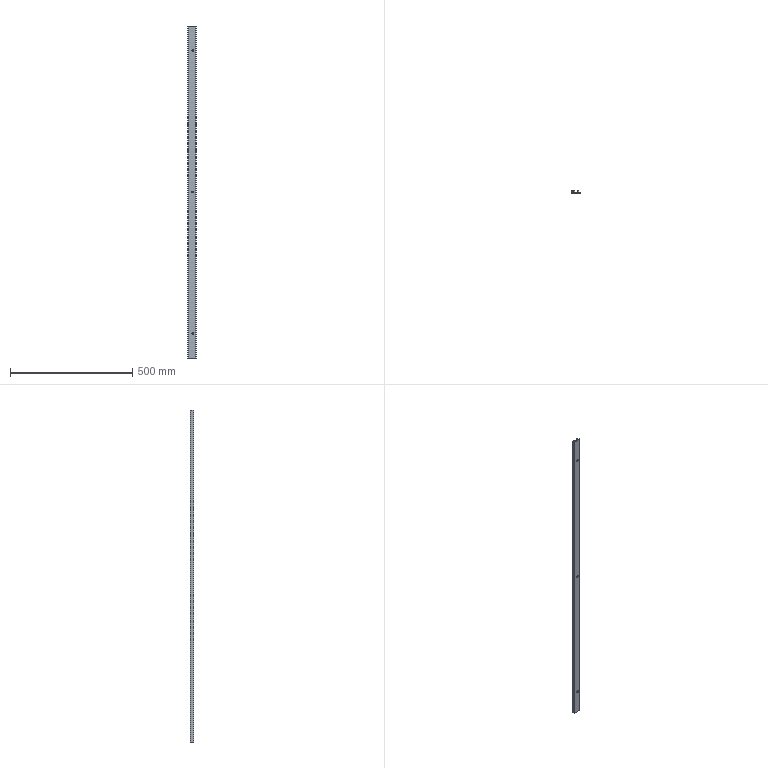Part | 1 solid | 31 faces | box 33.5 x 13.5 x 1360 mm | volume 254381 mm3 | plane 16 | cylinder 9 | cone 6 | commonest cylinder face diameters 2 x3 13.44 x3 4 x2 1.5 x1
STEP:
#1=CARTESIAN_POINT('',(20.,0.,1163.72));
#2=VERTEX_POINT('',#1);
#3=CARTESIAN_POINT('',(20.,0.,1156.28));
#4=VERTEX_POINT('',#3);
#5=CARTESIAN_POINT('',(20.,0.,1160.));
#6=DIRECTION('',(0.,-1.,0.));
#7=DIRECTION('',(0.,0.,-1.));
#8=AXIS2_PLACEMENT_3D('',#5,#6,#7);
#9=CIRCLE('',#8,3.72);
#10=EDGE_CURVE('',#2,#4,#9,.T.);
#11=ORIENTED_EDGE('',*,*,#10,.T.);
#12=CARTESIAN_POINT('',(20.,3.,1153.28));
#13=VERTEX_POINT('',#12);
#14=CARTESIAN_POINT('',(20.,3.,1153.28));
#15=DIRECTION('',(0.,0.7071,-0.7071));
#16=VECTOR('',#15,1000.);
#17=LINE('',#14,#16);
#18=EDGE_CURVE('',#4,#13,#17,.T.);
#19=ORIENTED_EDGE('',*,*,#18,.T.);
#20=CARTESIAN_POINT('',(20.,3.,1166.72));
#21=VERTEX_POINT('',#20);
#22=CARTESIAN_POINT('',(20.,3.,1160.));
#23=DIRECTION('',(0.,1.,0.));
#24=DIRECTION('',(0.,0.,1.));
#25=AXIS2_PLACEMENT_3D('',#22,#23,#24);
#26=CIRCLE('',#25,6.72);
#27=EDGE_CURVE('',#13,#21,#26,.T.);
#28=ORIENTED_EDGE('',*,*,#27,.T.);
#29=CARTESIAN_POINT('',(20.,3.,1166.72));
#30=DIRECTION('',(0.,0.7071,0.7071));
#31=VECTOR('',#30,1000.);
#32=LINE('',#29,#31);
#33=EDGE_CURVE('',#2,#21,#32,.T.);
#34=ORIENTED_EDGE('',*,*,#33,.F.);
#35=EDGE_LOOP('',(#11,#19,#28,#34));
#36=FACE_OUTER_BOUND('',#35,.T.);
#37=CARTESIAN_POINT('',(20.,3.,1160.));
#38=DIRECTION('',(0.,1.,0.));
#39=DIRECTION('',(0.,0.,1.));
#40=AXIS2_PLACEMENT_3D('',#37,#38,#39);
#41=CONICAL_SURFACE('',#40,6.72,0.7854);
#42=ADVANCED_FACE('',(#36),#41,.F.);
#43=CARTESIAN_POINT('',(20.,0.,3.72));
#44=VERTEX_POINT('',#43);
#45=CARTESIAN_POINT('',(20.,0.,-3.72));
#46=VERTEX_POINT('',#45);
#47=CARTESIAN_POINT('',(20.,0.,0.));
#48=DIRECTION('',(0.,-1.,0.));
#49=DIRECTION('',(0.,0.,-1.));
#50=AXIS2_PLACEMENT_3D('',#47,#48,#49);
#51=CIRCLE('',#50,3.72);
#52=EDGE_CURVE('',#44,#46,#51,.T.);
#53=ORIENTED_EDGE('',*,*,#52,.T.);
#54=CARTESIAN_POINT('',(20.,3.,-6.72));
#55=VERTEX_POINT('',#54);
#56=CARTESIAN_POINT('',(20.,3.,-6.72));
#57=DIRECTION('',(0.,0.7071,-0.7071));
#58=VECTOR('',#57,1000.);
#59=LINE('',#56,#58);
#60=EDGE_CURVE('',#46,#55,#59,.T.);
#61=ORIENTED_EDGE('',*,*,#60,.T.);
#62=CARTESIAN_POINT('',(20.,3.,6.72));
#63=VERTEX_POINT('',#62);
#64=CARTESIAN_POINT('',(20.,3.,0.));
#65=DIRECTION('',(0.,1.,0.));
#66=DIRECTION('',(0.,0.,1.));
#67=AXIS2_PLACEMENT_3D('',#64,#65,#66);
#68=CIRCLE('',#67,6.72);
#69=EDGE_CURVE('',#55,#63,#68,.T.);
#70=ORIENTED_EDGE('',*,*,#69,.T.);
#71=CARTESIAN_POINT('',(20.,3.,6.72));
#72=DIRECTION('',(0.,0.7071,0.7071));
#73=VECTOR('',#72,1000.);
#74=LINE('',#71,#73);
#75=EDGE_CURVE('',#44,#63,#74,.T.);
#76=ORIENTED_EDGE('',*,*,#75,.F.);
#77=EDGE_LOOP('',(#53,#61,#70,#76));
#78=FACE_OUTER_BOUND('',#77,.T.);
#79=CARTESIAN_POINT('',(20.,3.,0.));
#80=DIRECTION('',(0.,1.,0.));
#81=DIRECTION('',(0.,0.,1.));
#82=AXIS2_PLACEMENT_3D('',#79,#80,#81);
#83=CONICAL_SURFACE('',#82,6.72,0.7854);
#84=ADVANCED_FACE('',(#78),#83,.F.);
#85=CARTESIAN_POINT('',(20.,0.,583.72));
#86=VERTEX_POINT('',#85);
#87=CARTESIAN_POINT('',(20.,0.,576.28));
#88=VERTEX_POINT('',#87);
#89=CARTESIAN_POINT('',(20.,0.,580.));
#90=DIRECTION('',(0.,-1.,0.));
#91=DIRECTION('',(0.,0.,-1.));
#92=AXIS2_PLACEMENT_3D('',#89,#90,#91);
#93=CIRCLE('',#92,3.72);
#94=EDGE_CURVE('',#86,#88,#93,.T.);
#95=ORIENTED_EDGE('',*,*,#94,.T.);
#96=CARTESIAN_POINT('',(20.,3.,573.28));
#97=VERTEX_POINT('',#96);
#98=CARTESIAN_POINT('',(20.,3.,573.28));
#99=DIRECTION('',(0.,0.7071,-0.7071));
#100=VECTOR('',#99,1000.);
#101=LINE('',#98,#100);
#102=EDGE_CURVE('',#88,#97,#101,.T.);
#103=ORIENTED_EDGE('',*,*,#102,.T.);
#104=CARTESIAN_POINT('',(20.,3.,586.72));
#105=VERTEX_POINT('',#104);
#106=CARTESIAN_POINT('',(20.,3.,580.));
#107=DIRECTION('',(0.,1.,0.));
#108=DIRECTION('',(0.,0.,1.));
#109=AXIS2_PLACEMENT_3D('',#106,#107,#108);
#110=CIRCLE('',#109,6.72);
#111=EDGE_CURVE('',#97,#105,#110,.T.);
#112=ORIENTED_EDGE('',*,*,#111,.T.);
#113=CARTESIAN_POINT('',(20.,3.,586.72));
#114=DIRECTION('',(0.,0.7071,0.7071));
#115=VECTOR('',#114,1000.);
#116=LINE('',#113,#115);
#117=EDGE_CURVE('',#86,#105,#116,.T.);
#118=ORIENTED_EDGE('',*,*,#117,.F.);
#119=EDGE_LOOP('',(#95,#103,#112,#118));
#120=FACE_OUTER_BOUND('',#119,.T.);
#121=CARTESIAN_POINT('',(20.,3.,580.));
#122=DIRECTION('',(0.,1.,0.));
#123=DIRECTION('',(0.,0.,1.));
#124=AXIS2_PLACEMENT_3D('',#121,#122,#123);
#125=CONICAL_SURFACE('',#124,6.72,0.7854);
#126=ADVANCED_FACE('',(#120),#125,.F.);
#127=CARTESIAN_POINT('',(24.5,10.5,-4.991));
#128=VERTEX_POINT('',#127);
#129=CARTESIAN_POINT('',(24.5,10.5,-100.));
#130=VERTEX_POINT('',#129);
#131=CARTESIAN_POINT('',(24.5,10.5,-100.));
#132=DIRECTION('',(0.,0.,-1.));
#133=VECTOR('',#132,1000.);
#134=LINE('',#131,#133);
#135=EDGE_CURVE('',#128,#130,#134,.T.);
#136=ORIENTED_EDGE('',*,*,#135,.F.);
#137=CARTESIAN_POINT('',(24.5,10.5,4.991));
#138=VERTEX_POINT('',#137);
#139=CARTESIAN_POINT('',(24.5,10.5,-4.991));
#140=CARTESIAN_POINT('',(24.5,10.638,-4.991));
#141=CARTESIAN_POINT('',(24.515,10.777,-4.978));
#142=CARTESIAN_POINT('',(24.57,11.043,-4.927));
#143=CARTESIAN_POINT('',(24.611,11.171,-4.889));
#144=CARTESIAN_POINT('',(24.765,11.529,-4.74));
#145=CARTESIAN_POINT('',(24.907,11.728,-4.597));
#146=CARTESIAN_POINT('',(25.205,12.04,-4.256));
#147=CARTESIAN_POINT('',(25.365,12.156,-4.055));
#148=CARTESIAN_POINT('',(25.663,12.325,-3.627));
#149=CARTESIAN_POINT('',(25.806,12.38,-3.395));
#150=CARTESIAN_POINT('',(26.19,12.494,-2.672));
#151=CARTESIAN_POINT('',(26.387,12.501,-2.161));
#152=CARTESIAN_POINT('',(26.654,12.499,-1.091));
#153=CARTESIAN_POINT('',(26.72,12.488,-0.5481));
#154=CARTESIAN_POINT('',(26.72,12.488,0.2773));
#155=CARTESIAN_POINT('',(26.703,12.49,0.5529));
#156=CARTESIAN_POINT('',(26.636,12.496,1.095));
#157=CARTESIAN_POINT('',(26.586,12.499,1.362));
#158=CARTESIAN_POINT('',(26.388,12.501,2.155));
#159=CARTESIAN_POINT('',(26.188,12.493,2.677));
#160=CARTESIAN_POINT('',(25.805,12.38,3.396));
#161=CARTESIAN_POINT('',(25.662,12.324,3.629));
#162=CARTESIAN_POINT('',(25.438,12.197,3.95));
#163=CARTESIAN_POINT('',(25.362,12.147,4.053));
#164=CARTESIAN_POINT('',(25.208,12.03,4.249));
#165=CARTESIAN_POINT('',(25.13,11.961,4.342));
#166=CARTESIAN_POINT('',(24.98,11.805,4.513));
#167=CARTESIAN_POINT('',(24.908,11.717,4.591));
#168=CARTESIAN_POINT('',(24.774,11.518,4.73));
#169=CARTESIAN_POINT('',(24.714,11.408,4.79));
#170=CARTESIAN_POINT('',(24.612,11.172,4.888));
#171=CARTESIAN_POINT('',(24.57,11.043,4.927));
#172=CARTESIAN_POINT('',(24.515,10.778,4.978));
#173=CARTESIAN_POINT('',(24.5,10.64,4.991));
#174=CARTESIAN_POINT('',(24.5,10.5,4.991));
#175=B_SPLINE_CURVE_WITH_KNOTS('',3,(#139,#140,#141,#142,#143,#144,#145,#146,#147,#148,#149,#150,#151,#152,#153,#154,#155,#156,#157,#158,#159,#160,#161,#162,#163,#164,#165,#166,#167,#168,#169,#170,#171,#172,#173,#174),.UNSPECIFIED.,.F.,.F.,(4,2,2,2,2,2,2,2,2,2,2,2,2,2,2,2,2,4),(0.01321,0.01362,0.01403,0.01486,0.01569,0.01651,0.01816,0.01981,0.02064,0.02146,0.02311,0.02394,0.02435,0.02477,0.02518,0.02559,0.026,0.02642),.UNSPECIFIED.);
#176=EDGE_CURVE('',#128,#138,#175,.T.);
#177=ORIENTED_EDGE('',*,*,#176,.T.);
#178=CARTESIAN_POINT('',(24.5,10.5,575.009));
#179=VERTEX_POINT('',#178);
#180=CARTESIAN_POINT('',(24.5,10.5,-100.));
#181=DIRECTION('',(0.,0.,-1.));
#182=VECTOR('',#181,1000.);
#183=LINE('',#180,#182);
#184=EDGE_CURVE('',#179,#138,#183,.T.);
#185=ORIENTED_EDGE('',*,*,#184,.F.);
#186=CARTESIAN_POINT('',(24.5,10.5,584.991));
#187=VERTEX_POINT('',#186);
#188=CARTESIAN_POINT('',(24.5,10.5,575.009));
#189=CARTESIAN_POINT('',(24.5,10.638,575.009));
#190=CARTESIAN_POINT('',(24.515,10.777,575.022));
#191=CARTESIAN_POINT('',(24.57,11.043,575.073));
#192=CARTESIAN_POINT('',(24.611,11.171,575.111));
#193=CARTESIAN_POINT('',(24.765,11.529,575.26));
#194=CARTESIAN_POINT('',(24.907,11.728,575.403));
#195=CARTESIAN_POINT('',(25.205,12.04,575.744));
#196=CARTESIAN_POINT('',(25.365,12.156,575.945));
#197=CARTESIAN_POINT('',(25.663,12.325,576.373));
#198=CARTESIAN_POINT('',(25.806,12.38,576.605));
#199=CARTESIAN_POINT('',(26.19,12.494,577.328));
#200=CARTESIAN_POINT('',(26.387,12.501,577.839));
#201=CARTESIAN_POINT('',(26.654,12.499,578.909));
#202=CARTESIAN_POINT('',(26.72,12.488,579.452));
#203=CARTESIAN_POINT('',(26.72,12.488,580.277));
#204=CARTESIAN_POINT('',(26.703,12.49,580.553));
#205=CARTESIAN_POINT('',(26.636,12.496,581.095));
#206=CARTESIAN_POINT('',(26.586,12.499,581.362));
#207=CARTESIAN_POINT('',(26.388,12.501,582.155));
#208=CARTESIAN_POINT('',(26.188,12.493,582.677));
#209=CARTESIAN_POINT('',(25.805,12.38,583.396));
#210=CARTESIAN_POINT('',(25.662,12.324,583.629));
#211=CARTESIAN_POINT('',(25.438,12.197,583.95));
#212=CARTESIAN_POINT('',(25.362,12.147,584.053));
#213=CARTESIAN_POINT('',(25.208,12.03,584.249));
#214=CARTESIAN_POINT('',(25.13,11.961,584.342));
#215=CARTESIAN_POINT('',(24.98,11.805,584.513));
#216=CARTESIAN_POINT('',(24.908,11.717,584.591));
#217=CARTESIAN_POINT('',(24.774,11.518,584.73));
#218=CARTESIAN_POINT('',(24.714,11.408,584.79));
#219=CARTESIAN_POINT('',(24.612,11.172,584.888));
#220=CARTESIAN_POINT('',(24.57,11.043,584.927));
#221=CARTESIAN_POINT('',(24.515,10.778,584.978));
#222=CARTESIAN_POINT('',(24.5,10.64,584.991));
#223=CARTESIAN_POINT('',(24.5,10.5,584.991));
#224=B_SPLINE_CURVE_WITH_KNOTS('',3,(#188,#189,#190,#191,#192,#193,#194,#195,#196,#197,#198,#199,#200,#201,#202,#203,#204,#205,#206,#207,#208,#209,#210,#211,#212,#213,#214,#215,#216,#217,#218,#219,#220,#221,#222,#223),.UNSPECIFIED.,.F.,.F.,(4,2,2,2,2,2,2,2,2,2,2,2,2,2,2,2,2,4),(0.01321,0.01362,0.01403,0.01486,0.01569,0.01651,0.01816,0.01981,0.02064,0.02146,0.02311,0.02394,0.02435,0.02477,0.02518,0.02559,0.026,0.02642),.UNSPECIFIED.);
#225=EDGE_CURVE('',#179,#187,#224,.T.);
#226=ORIENTED_EDGE('',*,*,#225,.T.);
#227=CARTESIAN_POINT('',(24.5,10.5,1155.009));
#228=VERTEX_POINT('',#227);
#229=CARTESIAN_POINT('',(24.5,10.5,-100.));
#230=DIRECTION('',(0.,0.,-1.));
#231=VECTOR('',#230,1000.);
#232=LINE('',#229,#231);
#233=EDGE_CURVE('',#228,#187,#232,.T.);
#234=ORIENTED_EDGE('',*,*,#233,.F.);
#235=CARTESIAN_POINT('',(24.5,10.5,1164.991));
#236=VERTEX_POINT('',#235);
#237=CARTESIAN_POINT('',(24.5,10.5,1155.009));
#238=CARTESIAN_POINT('',(24.5,10.64,1155.009));
#239=CARTESIAN_POINT('',(24.514,10.776,1155.022));
#240=CARTESIAN_POINT('',(24.57,11.042,1155.073));
#241=CARTESIAN_POINT('',(24.611,11.171,1155.111));
#242=CARTESIAN_POINT('',(24.713,11.408,1155.209));
#243=CARTESIAN_POINT('',(24.775,11.519,1155.27));
#244=CARTESIAN_POINT('',(24.908,11.717,1155.409));
#245=CARTESIAN_POINT('',(24.981,11.806,1155.488));
#246=CARTESIAN_POINT('',(25.207,12.042,1155.746));
#247=CARTESIAN_POINT('',(25.363,12.155,1155.942));
#248=CARTESIAN_POINT('',(25.665,12.326,1156.376));
#249=CARTESIAN_POINT('',(25.806,12.38,1156.605));
#250=CARTESIAN_POINT('',(26.061,12.456,1157.084));
#251=CARTESIAN_POINT('',(26.176,12.476,1157.337));
#252=CARTESIAN_POINT('',(26.372,12.498,1157.849));
#253=CARTESIAN_POINT('',(26.454,12.501,1158.109));
#254=CARTESIAN_POINT('',(26.586,12.499,1158.638));
#255=CARTESIAN_POINT('',(26.636,12.496,1158.907));
#256=CARTESIAN_POINT('',(26.703,12.49,1159.453));
#257=CARTESIAN_POINT('',(26.72,12.488,1159.729));
#258=CARTESIAN_POINT('',(26.72,12.488,1160.275));
#259=CARTESIAN_POINT('',(26.703,12.49,1160.547));
#260=CARTESIAN_POINT('',(26.637,12.496,1161.089));
#261=CARTESIAN_POINT('',(26.587,12.499,1161.36));
#262=CARTESIAN_POINT('',(26.387,12.501,1162.161));
#263=CARTESIAN_POINT('',(26.191,12.494,1162.671));
#264=CARTESIAN_POINT('',(25.805,12.38,1163.396));
#265=CARTESIAN_POINT('',(25.663,12.325,1163.627));
#266=CARTESIAN_POINT('',(25.364,12.155,1164.057));
#267=CARTESIAN_POINT('',(25.205,12.039,1164.256));
#268=CARTESIAN_POINT('',(24.981,11.805,1164.512));
#269=CARTESIAN_POINT('',(24.907,11.716,1164.592));
#270=CARTESIAN_POINT('',(24.774,11.518,1164.73));
#271=CARTESIAN_POINT('',(24.714,11.409,1164.79));
#272=CARTESIAN_POINT('',(24.611,11.17,1164.889));
#273=CARTESIAN_POINT('',(24.571,11.044,1164.926));
#274=CARTESIAN_POINT('',(24.515,10.78,1164.977));
#275=CARTESIAN_POINT('',(24.5,10.64,1164.991));
#276=CARTESIAN_POINT('',(24.5,10.5,1164.991));
#277=B_SPLINE_CURVE_WITH_KNOTS('',3,(#237,#238,#239,#240,#241,#242,#243,#244,#245,#246,#247,#248,#249,#250,#251,#252,#253,#254,#255,#256,#257,#258,#259,#260,#261,#262,#263,#264,#265,#266,#267,#268,#269,#270,#271,#272,#273,#274,#275,#276),.UNSPECIFIED.,.F.,.F.,(4,2,2,2,2,2,2,2,2,2,2,2,2,2,2,2,2,2,2,4),(0.,0.0004127,0.0008255,0.001238,0.001651,0.002476,0.003302,0.004127,0.004953,0.005778,0.006604,0.007429,0.008255,0.009906,0.01073,0.01156,0.01197,0.01238,0.01279,0.01321),.UNSPECIFIED.);
#278=EDGE_CURVE('',#228,#236,#277,.T.);
#279=ORIENTED_EDGE('',*,*,#278,.T.);
#280=CARTESIAN_POINT('',(24.5,10.5,1260.));
#281=VERTEX_POINT('',#280);
#282=CARTESIAN_POINT('',(24.5,10.5,-100.));
#283=DIRECTION('',(0.,0.,-1.));
#284=VECTOR('',#283,1000.);
#285=LINE('',#282,#284);
#286=EDGE_CURVE('',#281,#236,#285,.T.);
#287=ORIENTED_EDGE('',*,*,#286,.F.);
#288=CARTESIAN_POINT('',(28.5,10.5,1260.));
#289=VERTEX_POINT('',#288);
#290=CARTESIAN_POINT('',(26.5,10.5,1260.));
#291=DIRECTION('',(0.,0.,1.));
#292=DIRECTION('',(1.,0.,0.));
#293=AXIS2_PLACEMENT_3D('',#290,#291,#292);
#294=CIRCLE('',#293,2.);
#295=EDGE_CURVE('',#289,#281,#294,.T.);
#296=ORIENTED_EDGE('',*,*,#295,.F.);
#297=CARTESIAN_POINT('',(28.5,10.5,-100.));
#298=VERTEX_POINT('',#297);
#299=CARTESIAN_POINT('',(28.5,10.5,-100.));
#300=DIRECTION('',(0.,0.,-1.));
#301=VECTOR('',#300,1000.);
#302=LINE('',#299,#301);
#303=EDGE_CURVE('',#289,#298,#302,.T.);
#304=ORIENTED_EDGE('',*,*,#303,.T.);
#305=CARTESIAN_POINT('',(26.5,10.5,-100.));
#306=DIRECTION('',(0.,0.,1.));
#307=DIRECTION('',(-1.,0.,0.));
#308=AXIS2_PLACEMENT_3D('',#305,#306,#307);
#309=CIRCLE('',#308,2.);
#310=EDGE_CURVE('',#298,#130,#309,.T.);
#311=ORIENTED_EDGE('',*,*,#310,.T.);
#312=EDGE_LOOP('',(#136,#177,#185,#226,#234,#279,#287,#296,#304,#311));
#313=FACE_OUTER_BOUND('',#312,.T.);
#314=CARTESIAN_POINT('',(26.5,10.5,-100.));
#315=DIRECTION('',(0.,0.,-1.));
#316=DIRECTION('',(-1.,0.,0.));
#317=AXIS2_PLACEMENT_3D('',#314,#315,#316);
#318=CYLINDRICAL_SURFACE('',#317,2.);
#319=ADVANCED_FACE('',(#313),#318,.T.);
#320=CARTESIAN_POINT('',(24.5,3.,-4.991));
#321=VERTEX_POINT('',#320);
#322=CARTESIAN_POINT('',(24.5,3.,-100.));
#323=VERTEX_POINT('',#322);
#324=CARTESIAN_POINT('',(24.5,3.,-100.));
#325=DIRECTION('',(0.,0.,-1.));
#326=VECTOR('',#325,1000.);
#327=LINE('',#324,#326);
#328=EDGE_CURVE('',#321,#323,#327,.T.);
#329=ORIENTED_EDGE('',*,*,#328,.F.);
#330=CARTESIAN_POINT('',(24.5,13.5,-4.991));
#331=DIRECTION('',(0.,1.,0.));
#332=VECTOR('',#331,1000.);
#333=LINE('',#330,#332);
#334=EDGE_CURVE('',#321,#128,#333,.T.);
#335=ORIENTED_EDGE('',*,*,#334,.T.);
#336=ORIENTED_EDGE('',*,*,#135,.T.);
#337=CARTESIAN_POINT('',(24.5,1.,-100.));
#338=DIRECTION('',(0.,-1.,0.));
#339=VECTOR('',#338,1000.);
#340=LINE('',#337,#339);
#341=EDGE_CURVE('',#130,#323,#340,.T.);
#342=ORIENTED_EDGE('',*,*,#341,.T.);
#343=EDGE_LOOP('',(#329,#335,#336,#342));
#344=FACE_OUTER_BOUND('',#343,.T.);
#345=CARTESIAN_POINT('',(24.5,10.5,-100.));
#346=DIRECTION('',(-1.,0.,0.));
#347=DIRECTION('',(0.,0.,1.));
#348=AXIS2_PLACEMENT_3D('',#345,#346,#347);
#349=PLANE('',#348);
#350=ADVANCED_FACE('',(#344),#349,.T.);
#351=ORIENTED_EDGE('',*,*,#184,.T.);
#352=CARTESIAN_POINT('',(24.5,3.,4.991));
#353=VERTEX_POINT('',#352);
#354=CARTESIAN_POINT('',(24.5,13.5,4.991));
#355=DIRECTION('',(0.,-1.,0.));
#356=VECTOR('',#355,1000.);
#357=LINE('',#354,#356);
#358=EDGE_CURVE('',#138,#353,#357,.T.);
#359=ORIENTED_EDGE('',*,*,#358,.T.);
#360=CARTESIAN_POINT('',(24.5,3.,575.009));
#361=VERTEX_POINT('',#360);
#362=CARTESIAN_POINT('',(24.5,3.,-100.));
#363=DIRECTION('',(0.,0.,-1.));
#364=VECTOR('',#363,1000.);
#365=LINE('',#362,#364);
#366=EDGE_CURVE('',#361,#353,#365,.T.);
#367=ORIENTED_EDGE('',*,*,#366,.F.);
#368=CARTESIAN_POINT('',(24.5,13.5,575.009));
#369=DIRECTION('',(0.,1.,0.));
#370=VECTOR('',#369,1000.);
#371=LINE('',#368,#370);
#372=EDGE_CURVE('',#361,#179,#371,.T.);
#373=ORIENTED_EDGE('',*,*,#372,.T.);
#374=EDGE_LOOP('',(#351,#359,#367,#373));
#375=FACE_OUTER_BOUND('',#374,.T.);
#376=CARTESIAN_POINT('',(24.5,10.5,-100.));
#377=DIRECTION('',(-1.,0.,0.));
#378=DIRECTION('',(0.,0.,1.));
#379=AXIS2_PLACEMENT_3D('',#376,#377,#378);
#380=PLANE('',#379);
#381=ADVANCED_FACE('',(#375),#380,.T.);
#382=ORIENTED_EDGE('',*,*,#233,.T.);
#383=CARTESIAN_POINT('',(24.5,3.,584.991));
#384=VERTEX_POINT('',#383);
#385=CARTESIAN_POINT('',(24.5,13.5,584.991));
#386=DIRECTION('',(0.,-1.,0.));
#387=VECTOR('',#386,1000.);
#388=LINE('',#385,#387);
#389=EDGE_CURVE('',#187,#384,#388,.T.);
#390=ORIENTED_EDGE('',*,*,#389,.T.);
#391=CARTESIAN_POINT('',(24.5,3.,1155.009));
#392=VERTEX_POINT('',#391);
#393=CARTESIAN_POINT('',(24.5,3.,-100.));
#394=DIRECTION('',(0.,0.,-1.));
#395=VECTOR('',#394,1000.);
#396=LINE('',#393,#395);
#397=EDGE_CURVE('',#392,#384,#396,.T.);
#398=ORIENTED_EDGE('',*,*,#397,.F.);
#399=CARTESIAN_POINT('',(24.5,13.5,1155.009));
#400=DIRECTION('',(0.,1.,0.));
#401=VECTOR('',#400,1000.);
#402=LINE('',#399,#401);
#403=EDGE_CURVE('',#392,#228,#402,.T.);
#404=ORIENTED_EDGE('',*,*,#403,.T.);
#405=EDGE_LOOP('',(#382,#390,#398,#404));
#406=FACE_OUTER_BOUND('',#405,.T.);
#407=CARTESIAN_POINT('',(24.5,10.5,-100.));
#408=DIRECTION('',(-1.,0.,0.));
#409=DIRECTION('',(0.,0.,1.));
#410=AXIS2_PLACEMENT_3D('',#407,#408,#409);
#411=PLANE('',#410);
#412=ADVANCED_FACE('',(#406),#411,.T.);
#413=ORIENTED_EDGE('',*,*,#286,.T.);
#414=CARTESIAN_POINT('',(24.5,3.,1164.991));
#415=VERTEX_POINT('',#414);
#416=CARTESIAN_POINT('',(24.5,13.5,1164.991));
#417=DIRECTION('',(0.,-1.,0.));
#418=VECTOR('',#417,1000.);
#419=LINE('',#416,#418);
#420=EDGE_CURVE('',#236,#415,#419,.T.);
#421=ORIENTED_EDGE('',*,*,#420,.T.);
#422=CARTESIAN_POINT('',(24.5,3.,1260.));
#423=VERTEX_POINT('',#422);
#424=CARTESIAN_POINT('',(24.5,3.,-100.));
#425=DIRECTION('',(0.,0.,-1.));
#426=VECTOR('',#425,1000.);
#427=LINE('',#424,#426);
#428=EDGE_CURVE('',#423,#415,#427,.T.);
#429=ORIENTED_EDGE('',*,*,#428,.F.);
#430=CARTESIAN_POINT('',(24.5,1.,1260.));
#431=DIRECTION('',(0.,-1.,0.));
#432=VECTOR('',#431,1000.);
#433=LINE('',#430,#432);
#434=EDGE_CURVE('',#281,#423,#433,.T.);
#435=ORIENTED_EDGE('',*,*,#434,.F.);
#436=EDGE_LOOP('',(#413,#421,#429,#435));
#437=FACE_OUTER_BOUND('',#436,.T.);
#438=CARTESIAN_POINT('',(24.5,10.5,-100.));
#439=DIRECTION('',(-1.,0.,0.));
#440=DIRECTION('',(0.,0.,1.));
#441=AXIS2_PLACEMENT_3D('',#438,#439,#440);
#442=PLANE('',#441);
#443=ADVANCED_FACE('',(#437),#442,.T.);
#444=ORIENTED_EDGE('',*,*,#10,.F.);
#445=CARTESIAN_POINT('',(20.,0.,1160.));
#446=DIRECTION('',(0.,-1.,0.));
#447=DIRECTION('',(0.,0.,-1.));
#448=AXIS2_PLACEMENT_3D('',#445,#446,#447);
#449=CIRCLE('',#448,3.72);
#450=EDGE_CURVE('',#4,#2,#449,.T.);
#451=ORIENTED_EDGE('',*,*,#450,.F.);
#452=EDGE_LOOP('',(#444,#451));
#453=FACE_BOUND('',#452,.T.);
#454=ORIENTED_EDGE('',*,*,#52,.F.);
#455=CARTESIAN_POINT('',(20.,0.,0.));
#456=DIRECTION('',(0.,-1.,0.));
#457=DIRECTION('',(0.,0.,-1.));
#458=AXIS2_PLACEMENT_3D('',#455,#456,#457);
#459=CIRCLE('',#458,3.72);
#460=EDGE_CURVE('',#46,#44,#459,.T.);
#461=ORIENTED_EDGE('',*,*,#460,.F.);
#462=EDGE_LOOP('',(#454,#461));
#463=FACE_BOUND('',#462,.T.);
#464=CARTESIAN_POINT('',(1.,0.,-100.));
#465=VERTEX_POINT('',#464);
#466=CARTESIAN_POINT('',(32.5,0.,-100.));
#467=VERTEX_POINT('',#466);
#468=CARTESIAN_POINT('',(1.,0.,-100.));
#469=DIRECTION('',(1.,0.,0.));
#470=VECTOR('',#469,1000.);
#471=LINE('',#468,#470);
#472=EDGE_CURVE('',#465,#467,#471,.T.);
#473=ORIENTED_EDGE('',*,*,#472,.T.);
#474=CARTESIAN_POINT('',(32.5,0.,1260.));
#475=VERTEX_POINT('',#474);
#476=CARTESIAN_POINT('',(32.5,0.,-100.));
#477=DIRECTION('',(0.,0.,1.));
#478=VECTOR('',#477,1000.);
#479=LINE('',#476,#478);
#480=EDGE_CURVE('',#467,#475,#479,.T.);
#481=ORIENTED_EDGE('',*,*,#480,.T.);
#482=CARTESIAN_POINT('',(1.,0.,1260.));
#483=VERTEX_POINT('',#482);
#484=CARTESIAN_POINT('',(1.,0.,1260.));
#485=DIRECTION('',(-1.,0.,0.));
#486=VECTOR('',#485,1000.);
#487=LINE('',#484,#486);
#488=EDGE_CURVE('',#475,#483,#487,.T.);
#489=ORIENTED_EDGE('',*,*,#488,.T.);
#490=CARTESIAN_POINT('',(1.,0.,-100.));
#491=DIRECTION('',(0.,0.,-1.));
#492=VECTOR('',#491,1000.);
#493=LINE('',#490,#492);
#494=EDGE_CURVE('',#483,#465,#493,.T.);
#495=ORIENTED_EDGE('',*,*,#494,.T.);
#496=EDGE_LOOP('',(#473,#481,#489,#495));
#497=FACE_OUTER_BOUND('',#496,.T.);
#498=ORIENTED_EDGE('',*,*,#94,.F.);
#499=CARTESIAN_POINT('',(20.,0.,580.));
#500=DIRECTION('',(0.,-1.,0.));
#501=DIRECTION('',(0.,0.,-1.));
#502=AXIS2_PLACEMENT_3D('',#499,#500,#501);
#503=CIRCLE('',#502,3.72);
#504=EDGE_CURVE('',#88,#86,#503,.T.);
#505=ORIENTED_EDGE('',*,*,#504,.F.);
#506=EDGE_LOOP('',(#498,#505));
#507=FACE_BOUND('',#506,.T.);
#508=CARTESIAN_POINT('',(1.,0.,-100.));
#509=DIRECTION('',(0.,-1.,0.));
#510=DIRECTION('',(0.,0.,-1.));
#511=AXIS2_PLACEMENT_3D('',#508,#509,#510);
#512=PLANE('',#511);
#513=ADVANCED_FACE('',(#453,#463,#497,#507),#512,.T.);
#514=CARTESIAN_POINT('',(33.5,1.,-100.));
#515=VERTEX_POINT('',#514);
#516=CARTESIAN_POINT('',(32.5,1.,-100.));
#517=DIRECTION('',(0.,0.,1.));
#518=DIRECTION('',(-1.,0.,0.));
#519=AXIS2_PLACEMENT_3D('',#516,#517,#518);
#520=CIRCLE('',#519,1.);
#521=EDGE_CURVE('',#467,#515,#520,.T.);
#522=ORIENTED_EDGE('',*,*,#521,.T.);
#523=CARTESIAN_POINT('',(33.5,1.,1260.));
#524=VERTEX_POINT('',#523);
#525=CARTESIAN_POINT('',(33.5,1.,-100.));
#526=DIRECTION('',(0.,0.,1.));
#527=VECTOR('',#526,1000.);
#528=LINE('',#525,#527);
#529=EDGE_CURVE('',#515,#524,#528,.T.);
#530=ORIENTED_EDGE('',*,*,#529,.T.);
#531=CARTESIAN_POINT('',(32.5,1.,1260.));
#532=DIRECTION('',(0.,0.,-1.));
#533=DIRECTION('',(1.,0.,0.));
#534=AXIS2_PLACEMENT_3D('',#531,#532,#533);
#535=CIRCLE('',#534,1.);
#536=EDGE_CURVE('',#524,#475,#535,.T.);
#537=ORIENTED_EDGE('',*,*,#536,.T.);
#538=ORIENTED_EDGE('',*,*,#480,.F.);
#539=EDGE_LOOP('',(#522,#530,#537,#538));
#540=FACE_OUTER_BOUND('',#539,.T.);
#541=CARTESIAN_POINT('',(32.5,1.,-100.));
#542=DIRECTION('',(0.,0.,-1.));
#543=DIRECTION('',(-1.,0.,0.));
#544=AXIS2_PLACEMENT_3D('',#541,#542,#543);
#545=CYLINDRICAL_SURFACE('',#544,1.);
#546=ADVANCED_FACE('',(#540),#545,.T.);
#547=CARTESIAN_POINT('',(1.5,12.75,-100.));
#548=VERTEX_POINT('',#547);
#549=CARTESIAN_POINT('',(0.,12.75,-100.));
#550=VERTEX_POINT('',#549);
#551=CARTESIAN_POINT('',(0.75,12.75,-100.));
#552=DIRECTION('',(0.,0.,1.));
#553=DIRECTION('',(-1.,0.,0.));
#554=AXIS2_PLACEMENT_3D('',#551,#552,#553);
#555=CIRCLE('',#554,0.75);
#556=EDGE_CURVE('',#548,#550,#555,.T.);
#557=ORIENTED_EDGE('',*,*,#556,.F.);
#558=CARTESIAN_POINT('',(1.5,3.,-100.));
#559=VERTEX_POINT('',#558);
#560=CARTESIAN_POINT('',(1.5,1.,-100.));
#561=DIRECTION('',(0.,1.,0.));
#562=VECTOR('',#561,1000.);
#563=LINE('',#560,#562);
#564=EDGE_CURVE('',#559,#548,#563,.T.);
#565=ORIENTED_EDGE('',*,*,#564,.F.);
#566=CARTESIAN_POINT('',(8.5,3.,-100.));
#567=VERTEX_POINT('',#566);
#568=CARTESIAN_POINT('',(1.,3.,-100.));
#569=DIRECTION('',(-1.,0.,0.));
#570=VECTOR('',#569,1000.);
#571=LINE('',#568,#570);
#572=EDGE_CURVE('',#567,#559,#571,.T.);
#573=ORIENTED_EDGE('',*,*,#572,.F.);
#574=CARTESIAN_POINT('',(8.5,10.5,-100.));
#575=VERTEX_POINT('',#574);
#576=CARTESIAN_POINT('',(8.5,1.,-100.));
#577=DIRECTION('',(0.,-1.,0.));
#578=VECTOR('',#577,1000.);
#579=LINE('',#576,#578);
#580=EDGE_CURVE('',#575,#567,#579,.T.);
#581=ORIENTED_EDGE('',*,*,#580,.F.);
#582=CARTESIAN_POINT('',(12.5,10.5,-100.));
#583=VERTEX_POINT('',#582);
#584=CARTESIAN_POINT('',(10.5,10.5,-100.));
#585=DIRECTION('',(0.,0.,1.));
#586=DIRECTION('',(-1.,0.,0.));
#587=AXIS2_PLACEMENT_3D('',#584,#585,#586);
#588=CIRCLE('',#587,2.);
#589=EDGE_CURVE('',#583,#575,#588,.T.);
#590=ORIENTED_EDGE('',*,*,#589,.F.);
#591=CARTESIAN_POINT('',(12.5,3.,-100.));
#592=VERTEX_POINT('',#591);
#593=CARTESIAN_POINT('',(12.5,1.,-100.));
#594=DIRECTION('',(0.,1.,0.));
#595=VECTOR('',#594,1000.);
#596=LINE('',#593,#595);
#597=EDGE_CURVE('',#592,#583,#596,.T.);
#598=ORIENTED_EDGE('',*,*,#597,.F.);
#599=CARTESIAN_POINT('',(1.,3.,-100.));
#600=DIRECTION('',(-1.,0.,0.));
#601=VECTOR('',#600,1000.);
#602=LINE('',#599,#601);
#603=EDGE_CURVE('',#323,#592,#602,.T.);
#604=ORIENTED_EDGE('',*,*,#603,.F.);
#605=ORIENTED_EDGE('',*,*,#341,.F.);
#606=ORIENTED_EDGE('',*,*,#310,.F.);
#607=CARTESIAN_POINT('',(28.5,3.,-100.));
#608=VERTEX_POINT('',#607);
#609=CARTESIAN_POINT('',(28.5,1.,-100.));
#610=DIRECTION('',(0.,1.,0.));
#611=VECTOR('',#610,1000.);
#612=LINE('',#609,#611);
#613=EDGE_CURVE('',#608,#298,#612,.T.);
#614=ORIENTED_EDGE('',*,*,#613,.F.);
#615=CARTESIAN_POINT('',(32.5,3.,-100.));
#616=VERTEX_POINT('',#615);
#617=CARTESIAN_POINT('',(1.,3.,-100.));
#618=DIRECTION('',(-1.,0.,0.));
#619=VECTOR('',#618,1000.);
#620=LINE('',#617,#619);
#621=EDGE_CURVE('',#616,#608,#620,.T.);
#622=ORIENTED_EDGE('',*,*,#621,.F.);
#623=CARTESIAN_POINT('',(33.5,2.,-100.));
#624=VERTEX_POINT('',#623);
#625=CARTESIAN_POINT('',(32.5,2.,-100.));
#626=DIRECTION('',(0.,0.,1.));
#627=DIRECTION('',(-1.,0.,0.));
#628=AXIS2_PLACEMENT_3D('',#625,#626,#627);
#629=CIRCLE('',#628,1.);
#630=EDGE_CURVE('',#624,#616,#629,.T.);
#631=ORIENTED_EDGE('',*,*,#630,.F.);
#632=CARTESIAN_POINT('',(33.5,1.,-100.));
#633=DIRECTION('',(0.,1.,0.));
#634=VECTOR('',#633,1000.);
#635=LINE('',#632,#634);
#636=EDGE_CURVE('',#515,#624,#635,.T.);
#637=ORIENTED_EDGE('',*,*,#636,.F.);
#638=ORIENTED_EDGE('',*,*,#521,.F.);
#639=ORIENTED_EDGE('',*,*,#472,.F.);
#640=CARTESIAN_POINT('',(0.,1.,-100.));
#641=VERTEX_POINT('',#640);
#642=CARTESIAN_POINT('',(1.,1.,-100.));
#643=DIRECTION('',(0.,0.,1.));
#644=DIRECTION('',(-1.,0.,0.));
#645=AXIS2_PLACEMENT_3D('',#642,#643,#644);
#646=CIRCLE('',#645,1.);
#647=EDGE_CURVE('',#641,#465,#646,.T.);
#648=ORIENTED_EDGE('',*,*,#647,.F.);
#649=CARTESIAN_POINT('',(0.,1.,-100.));
#650=DIRECTION('',(0.,-1.,0.));
#651=VECTOR('',#650,1000.);
#652=LINE('',#649,#651);
#653=EDGE_CURVE('',#550,#641,#652,.T.);
#654=ORIENTED_EDGE('',*,*,#653,.F.);
#655=EDGE_LOOP('',(#557,#565,#573,#581,#590,#598,#604,#605,#606,#614,#622,#631,#637,#638,#639,#648,#654));
#656=FACE_OUTER_BOUND('',#655,.T.);
#657=CARTESIAN_POINT('',(1.,1.,-100.));
#658=DIRECTION('',(0.,0.,1.));
#659=DIRECTION('',(1.,0.,0.));
#660=AXIS2_PLACEMENT_3D('',#657,#658,#659);
#661=PLANE('',#660);
#662=ADVANCED_FACE('',(#656),#661,.F.);
#663=ORIENTED_EDGE('',*,*,#647,.T.);
#664=ORIENTED_EDGE('',*,*,#494,.F.);
#665=CARTESIAN_POINT('',(0.,1.,1260.));
#666=VERTEX_POINT('',#665);
#667=CARTESIAN_POINT('',(1.,1.,1260.));
#668=DIRECTION('',(0.,0.,-1.));
#669=DIRECTION('',(1.,0.,0.));
#670=AXIS2_PLACEMENT_3D('',#667,#668,#669);
#671=CIRCLE('',#670,1.);
#672=EDGE_CURVE('',#483,#666,#671,.T.);
#673=ORIENTED_EDGE('',*,*,#672,.T.);
#674=CARTESIAN_POINT('',(0.,1.,-100.));
#675=DIRECTION('',(0.,0.,-1.));
#676=VECTOR('',#675,1000.);
#677=LINE('',#674,#676);
#678=EDGE_CURVE('',#666,#641,#677,.T.);
#679=ORIENTED_EDGE('',*,*,#678,.T.);
#680=EDGE_LOOP('',(#663,#664,#673,#679));
#681=FACE_OUTER_BOUND('',#680,.T.);
#682=CARTESIAN_POINT('',(1.,1.,-100.));
#683=DIRECTION('',(0.,0.,-1.));
#684=DIRECTION('',(-1.,0.,0.));
#685=AXIS2_PLACEMENT_3D('',#682,#683,#684);
#686=CYLINDRICAL_SURFACE('',#685,1.);
#687=ADVANCED_FACE('',(#681),#686,.T.);
#688=CARTESIAN_POINT('',(1.5,3.,1260.));
#689=VERTEX_POINT('',#688);
#690=CARTESIAN_POINT('',(1.5,12.75,1260.));
#691=VERTEX_POINT('',#690);
#692=CARTESIAN_POINT('',(1.5,1.,1260.));
#693=DIRECTION('',(0.,1.,0.));
#694=VECTOR('',#693,1000.);
#695=LINE('',#692,#694);
#696=EDGE_CURVE('',#689,#691,#695,.T.);
#697=ORIENTED_EDGE('',*,*,#696,.T.);
#698=CARTESIAN_POINT('',(0.,12.75,1260.));
#699=VERTEX_POINT('',#698);
#700=CARTESIAN_POINT('',(0.75,12.75,1260.));
#701=DIRECTION('',(0.,0.,1.));
#702=DIRECTION('',(1.,0.,0.));
#703=AXIS2_PLACEMENT_3D('',#700,#701,#702);
#704=CIRCLE('',#703,0.75);
#705=EDGE_CURVE('',#691,#699,#704,.T.);
#706=ORIENTED_EDGE('',*,*,#705,.T.);
#707=CARTESIAN_POINT('',(0.,1.,1260.));
#708=DIRECTION('',(0.,-1.,0.));
#709=VECTOR('',#708,1000.);
#710=LINE('',#707,#709);
#711=EDGE_CURVE('',#699,#666,#710,.T.);
#712=ORIENTED_EDGE('',*,*,#711,.T.);
#713=ORIENTED_EDGE('',*,*,#672,.F.);
#714=ORIENTED_EDGE('',*,*,#488,.F.);
#715=ORIENTED_EDGE('',*,*,#536,.F.);
#716=CARTESIAN_POINT('',(33.5,2.,1260.));
#717=VERTEX_POINT('',#716);
#718=CARTESIAN_POINT('',(33.5,1.,1260.));
#719=DIRECTION('',(0.,1.,0.));
#720=VECTOR('',#719,1000.);
#721=LINE('',#718,#720);
#722=EDGE_CURVE('',#524,#717,#721,.T.);
#723=ORIENTED_EDGE('',*,*,#722,.T.);
#724=CARTESIAN_POINT('',(32.5,3.,1260.));
#725=VERTEX_POINT('',#724);
#726=CARTESIAN_POINT('',(32.5,2.,1260.));
#727=DIRECTION('',(0.,0.,-1.));
#728=DIRECTION('',(1.,0.,0.));
#729=AXIS2_PLACEMENT_3D('',#726,#727,#728);
#730=CIRCLE('',#729,1.);
#731=EDGE_CURVE('',#725,#717,#730,.T.);
#732=ORIENTED_EDGE('',*,*,#731,.F.);
#733=CARTESIAN_POINT('',(28.5,3.,1260.));
#734=VERTEX_POINT('',#733);
#735=CARTESIAN_POINT('',(1.,3.,1260.));
#736=DIRECTION('',(-1.,0.,0.));
#737=VECTOR('',#736,1000.);
#738=LINE('',#735,#737);
#739=EDGE_CURVE('',#725,#734,#738,.T.);
#740=ORIENTED_EDGE('',*,*,#739,.T.);
#741=CARTESIAN_POINT('',(28.5,1.,1260.));
#742=DIRECTION('',(0.,1.,0.));
#743=VECTOR('',#742,1000.);
#744=LINE('',#741,#743);
#745=EDGE_CURVE('',#734,#289,#744,.T.);
#746=ORIENTED_EDGE('',*,*,#745,.T.);
#747=ORIENTED_EDGE('',*,*,#295,.T.);
#748=ORIENTED_EDGE('',*,*,#434,.T.);
#749=CARTESIAN_POINT('',(12.5,3.,1260.));
#750=VERTEX_POINT('',#749);
#751=CARTESIAN_POINT('',(1.,3.,1260.));
#752=DIRECTION('',(-1.,0.,0.));
#753=VECTOR('',#752,1000.);
#754=LINE('',#751,#753);
#755=EDGE_CURVE('',#423,#750,#754,.T.);
#756=ORIENTED_EDGE('',*,*,#755,.T.);
#757=CARTESIAN_POINT('',(12.5,10.5,1260.));
#758=VERTEX_POINT('',#757);
#759=CARTESIAN_POINT('',(12.5,1.,1260.));
#760=DIRECTION('',(0.,1.,0.));
#761=VECTOR('',#760,1000.);
#762=LINE('',#759,#761);
#763=EDGE_CURVE('',#750,#758,#762,.T.);
#764=ORIENTED_EDGE('',*,*,#763,.T.);
#765=CARTESIAN_POINT('',(8.5,10.5,1260.));
#766=VERTEX_POINT('',#765);
#767=CARTESIAN_POINT('',(10.5,10.5,1260.));
#768=DIRECTION('',(0.,0.,1.));
#769=DIRECTION('',(1.,0.,0.));
#770=AXIS2_PLACEMENT_3D('',#767,#768,#769);
#771=CIRCLE('',#770,2.);
#772=EDGE_CURVE('',#758,#766,#771,.T.);
#773=ORIENTED_EDGE('',*,*,#772,.T.);
#774=CARTESIAN_POINT('',(8.5,3.,1260.));
#775=VERTEX_POINT('',#774);
#776=CARTESIAN_POINT('',(8.5,1.,1260.));
#777=DIRECTION('',(0.,-1.,0.));
#778=VECTOR('',#777,1000.);
#779=LINE('',#776,#778);
#780=EDGE_CURVE('',#766,#775,#779,.T.);
#781=ORIENTED_EDGE('',*,*,#780,.T.);
#782=CARTESIAN_POINT('',(1.,3.,1260.));
#783=DIRECTION('',(-1.,0.,0.));
#784=VECTOR('',#783,1000.);
#785=LINE('',#782,#784);
#786=EDGE_CURVE('',#775,#689,#785,.T.);
#787=ORIENTED_EDGE('',*,*,#786,.T.);
#788=EDGE_LOOP('',(#697,#706,#712,#713,#714,#715,#723,#732,#740,#746,#747,#748,#756,#764,#773,#781,#787));
#789=FACE_OUTER_BOUND('',#788,.T.);
#790=CARTESIAN_POINT('',(1.,1.,1260.));
#791=DIRECTION('',(0.,0.,1.));
#792=DIRECTION('',(1.,0.,0.));
#793=AXIS2_PLACEMENT_3D('',#790,#791,#792);
#794=PLANE('',#793);
#795=ADVANCED_FACE('',(#789),#794,.T.);
#796=ORIENTED_EDGE('',*,*,#636,.T.);
#797=CARTESIAN_POINT('',(33.5,2.,-100.));
#798=DIRECTION('',(0.,0.,1.));
#799=VECTOR('',#798,1000.);
#800=LINE('',#797,#799);
#801=EDGE_CURVE('',#624,#717,#800,.T.);
#802=ORIENTED_EDGE('',*,*,#801,.T.);
#803=ORIENTED_EDGE('',*,*,#722,.F.);
#804=ORIENTED_EDGE('',*,*,#529,.F.);
#805=EDGE_LOOP('',(#796,#802,#803,#804));
#806=FACE_OUTER_BOUND('',#805,.T.);
#807=CARTESIAN_POINT('',(33.5,1.,-100.));
#808=DIRECTION('',(1.,0.,0.));
#809=DIRECTION('',(0.,0.,-1.));
#810=AXIS2_PLACEMENT_3D('',#807,#808,#809);
#811=PLANE('',#810);
#812=ADVANCED_FACE('',(#806),#811,.T.);
#813=ORIENTED_EDGE('',*,*,#653,.T.);
#814=ORIENTED_EDGE('',*,*,#678,.F.);
#815=ORIENTED_EDGE('',*,*,#711,.F.);
#816=CARTESIAN_POINT('',(0.,12.75,-100.));
#817=DIRECTION('',(0.,0.,-1.));
#818=VECTOR('',#817,1000.);
#819=LINE('',#816,#818);
#820=EDGE_CURVE('',#699,#550,#819,.T.);
#821=ORIENTED_EDGE('',*,*,#820,.T.);
#822=EDGE_LOOP('',(#813,#814,#815,#821));
#823=FACE_OUTER_BOUND('',#822,.T.);
#824=CARTESIAN_POINT('',(0.,12.75,-100.));
#825=DIRECTION('',(-1.,0.,0.));
#826=DIRECTION('',(0.,0.,1.));
#827=AXIS2_PLACEMENT_3D('',#824,#825,#826);
#828=PLANE('',#827);
#829=ADVANCED_FACE('',(#823),#828,.T.);
#830=ORIENTED_EDGE('',*,*,#556,.T.);
#831=ORIENTED_EDGE('',*,*,#820,.F.);
#832=ORIENTED_EDGE('',*,*,#705,.F.);
#833=CARTESIAN_POINT('',(1.5,12.75,-100.));
#834=DIRECTION('',(0.,0.,-1.));
#835=VECTOR('',#834,1000.);
#836=LINE('',#833,#835);
#837=EDGE_CURVE('',#691,#548,#836,.T.);
#838=ORIENTED_EDGE('',*,*,#837,.T.);
#839=EDGE_LOOP('',(#830,#831,#832,#838));
#840=FACE_OUTER_BOUND('',#839,.T.);
#841=CARTESIAN_POINT('',(0.75,12.75,-100.));
#842=DIRECTION('',(0.,0.,-1.));
#843=DIRECTION('',(-1.,0.,0.));
#844=AXIS2_PLACEMENT_3D('',#841,#842,#843);
#845=CYLINDRICAL_SURFACE('',#844,0.75);
#846=ADVANCED_FACE('',(#840),#845,.T.);
#847=ORIENTED_EDGE('',*,*,#564,.T.);
#848=ORIENTED_EDGE('',*,*,#837,.F.);
#849=ORIENTED_EDGE('',*,*,#696,.F.);
#850=CARTESIAN_POINT('',(1.5,3.,-100.));
#851=DIRECTION('',(0.,0.,-1.));
#852=VECTOR('',#851,1000.);
#853=LINE('',#850,#852);
#854=EDGE_CURVE('',#689,#559,#853,.T.);
#855=ORIENTED_EDGE('',*,*,#854,.T.);
#856=EDGE_LOOP('',(#847,#848,#849,#855));
#857=FACE_OUTER_BOUND('',#856,.T.);
#858=CARTESIAN_POINT('',(1.5,3.,-100.));
#859=DIRECTION('',(1.,0.,0.));
#860=DIRECTION('',(0.,0.,-1.));
#861=AXIS2_PLACEMENT_3D('',#858,#859,#860);
#862=PLANE('',#861);
#863=ADVANCED_FACE('',(#857),#862,.T.);
#864=ORIENTED_EDGE('',*,*,#572,.T.);
#865=ORIENTED_EDGE('',*,*,#854,.F.);
#866=ORIENTED_EDGE('',*,*,#786,.F.);
#867=CARTESIAN_POINT('',(8.5,3.,-100.));
#868=DIRECTION('',(0.,0.,-1.));
#869=VECTOR('',#868,1000.);
#870=LINE('',#867,#869);
#871=EDGE_CURVE('',#775,#567,#870,.T.);
#872=ORIENTED_EDGE('',*,*,#871,.T.);
#873=EDGE_LOOP('',(#864,#865,#866,#872));
#874=FACE_OUTER_BOUND('',#873,.T.);
#875=CARTESIAN_POINT('',(8.5,3.,-100.));
#876=DIRECTION('',(0.,1.,0.));
#877=DIRECTION('',(0.,0.,1.));
#878=AXIS2_PLACEMENT_3D('',#875,#876,#877);
#879=PLANE('',#878);
#880=ADVANCED_FACE('',(#874),#879,.T.);
#881=ORIENTED_EDGE('',*,*,#580,.T.);
#882=ORIENTED_EDGE('',*,*,#871,.F.);
#883=ORIENTED_EDGE('',*,*,#780,.F.);
#884=CARTESIAN_POINT('',(8.5,10.5,-100.));
#885=DIRECTION('',(0.,0.,-1.));
#886=VECTOR('',#885,1000.);
#887=LINE('',#884,#886);
#888=EDGE_CURVE('',#766,#575,#887,.T.);
#889=ORIENTED_EDGE('',*,*,#888,.T.);
#890=EDGE_LOOP('',(#881,#882,#883,#889));
#891=FACE_OUTER_BOUND('',#890,.T.);
#892=CARTESIAN_POINT('',(8.5,10.5,-100.));
#893=DIRECTION('',(-1.,0.,0.));
#894=DIRECTION('',(0.,0.,1.));
#895=AXIS2_PLACEMENT_3D('',#892,#893,#894);
#896=PLANE('',#895);
#897=ADVANCED_FACE('',(#891),#896,.T.);
#898=ORIENTED_EDGE('',*,*,#589,.T.);
#899=ORIENTED_EDGE('',*,*,#888,.F.);
#900=ORIENTED_EDGE('',*,*,#772,.F.);
#901=CARTESIAN_POINT('',(12.5,10.5,-100.));
#902=DIRECTION('',(0.,0.,-1.));
#903=VECTOR('',#902,1000.);
#904=LINE('',#901,#903);
#905=EDGE_CURVE('',#758,#583,#904,.T.);
#906=ORIENTED_EDGE('',*,*,#905,.T.);
#907=EDGE_LOOP('',(#898,#899,#900,#906));
#908=FACE_OUTER_BOUND('',#907,.T.);
#909=CARTESIAN_POINT('',(10.5,10.5,-100.));
#910=DIRECTION('',(0.,0.,-1.));
#911=DIRECTION('',(-1.,0.,0.));
#912=AXIS2_PLACEMENT_3D('',#909,#910,#911);
#913=CYLINDRICAL_SURFACE('',#912,2.);
#914=ADVANCED_FACE('',(#908),#913,.T.);
#915=ORIENTED_EDGE('',*,*,#597,.T.);
#916=ORIENTED_EDGE('',*,*,#905,.F.);
#917=ORIENTED_EDGE('',*,*,#763,.F.);
#918=CARTESIAN_POINT('',(12.5,3.,-100.));
#919=DIRECTION('',(0.,0.,-1.));
#920=VECTOR('',#919,1000.);
#921=LINE('',#918,#920);
#922=EDGE_CURVE('',#750,#592,#921,.T.);
#923=ORIENTED_EDGE('',*,*,#922,.T.);
#924=EDGE_LOOP('',(#915,#916,#917,#923));
#925=FACE_OUTER_BOUND('',#924,.T.);
#926=CARTESIAN_POINT('',(12.5,3.,-100.));
#927=DIRECTION('',(1.,0.,0.));
#928=DIRECTION('',(0.,0.,-1.));
#929=AXIS2_PLACEMENT_3D('',#926,#927,#928);
#930=PLANE('',#929);
#931=ADVANCED_FACE('',(#925),#930,.T.);
#932=CARTESIAN_POINT('',(20.,3.,1160.));
#933=DIRECTION('',(0.,1.,0.));
#934=DIRECTION('',(0.,0.,1.));
#935=AXIS2_PLACEMENT_3D('',#932,#933,#934);
#936=CIRCLE('',#935,6.72);
#937=EDGE_CURVE('',#392,#13,#936,.T.);
#938=ORIENTED_EDGE('',*,*,#937,.F.);
#939=ORIENTED_EDGE('',*,*,#397,.T.);
#940=CARTESIAN_POINT('',(20.,3.,580.));
#941=DIRECTION('',(0.,1.,0.));
#942=DIRECTION('',(0.,0.,1.));
#943=AXIS2_PLACEMENT_3D('',#940,#941,#942);
#944=CIRCLE('',#943,6.72);
#945=EDGE_CURVE('',#105,#384,#944,.T.);
#946=ORIENTED_EDGE('',*,*,#945,.F.);
#947=ORIENTED_EDGE('',*,*,#111,.F.);
#948=CARTESIAN_POINT('',(20.,3.,580.));
#949=DIRECTION('',(0.,1.,0.));
#950=DIRECTION('',(0.,0.,1.));
#951=AXIS2_PLACEMENT_3D('',#948,#949,#950);
#952=CIRCLE('',#951,6.72);
#953=EDGE_CURVE('',#361,#97,#952,.T.);
#954=ORIENTED_EDGE('',*,*,#953,.F.);
#955=ORIENTED_EDGE('',*,*,#366,.T.);
#956=CARTESIAN_POINT('',(20.,3.,0.));
#957=DIRECTION('',(0.,1.,0.));
#958=DIRECTION('',(0.,0.,1.));
#959=AXIS2_PLACEMENT_3D('',#956,#957,#958);
#960=CIRCLE('',#959,6.72);
#961=EDGE_CURVE('',#63,#353,#960,.T.);
#962=ORIENTED_EDGE('',*,*,#961,.F.);
#963=ORIENTED_EDGE('',*,*,#69,.F.);
#964=CARTESIAN_POINT('',(20.,3.,0.));
#965=DIRECTION('',(0.,1.,0.));
#966=DIRECTION('',(0.,0.,1.));
#967=AXIS2_PLACEMENT_3D('',#964,#965,#966);
#968=CIRCLE('',#967,6.72);
#969=EDGE_CURVE('',#321,#55,#968,.T.);
#970=ORIENTED_EDGE('',*,*,#969,.F.);
#971=ORIENTED_EDGE('',*,*,#328,.T.);
#972=ORIENTED_EDGE('',*,*,#603,.T.);
#973=ORIENTED_EDGE('',*,*,#922,.F.);
#974=ORIENTED_EDGE('',*,*,#755,.F.);
#975=ORIENTED_EDGE('',*,*,#428,.T.);
#976=CARTESIAN_POINT('',(20.,3.,1160.));
#977=DIRECTION('',(0.,1.,0.));
#978=DIRECTION('',(0.,0.,1.));
#979=AXIS2_PLACEMENT_3D('',#976,#977,#978);
#980=CIRCLE('',#979,6.72);
#981=EDGE_CURVE('',#21,#415,#980,.T.);
#982=ORIENTED_EDGE('',*,*,#981,.F.);
#983=ORIENTED_EDGE('',*,*,#27,.F.);
#984=EDGE_LOOP('',(#938,#939,#946,#947,#954,#955,#962,#963,#970,#971,#972,#973,#974,#975,#982,#983));
#985=FACE_OUTER_BOUND('',#984,.T.);
#986=CARTESIAN_POINT('',(24.5,3.,-100.));
#987=DIRECTION('',(0.,1.,0.));
#988=DIRECTION('',(0.,0.,1.));
#989=AXIS2_PLACEMENT_3D('',#986,#987,#988);
#990=PLANE('',#989);
#991=ADVANCED_FACE('',(#985),#990,.T.);
#992=ORIENTED_EDGE('',*,*,#613,.T.);
#993=ORIENTED_EDGE('',*,*,#303,.F.);
#994=ORIENTED_EDGE('',*,*,#745,.F.);
#995=CARTESIAN_POINT('',(28.5,3.,-100.));
#996=DIRECTION('',(0.,0.,-1.));
#997=VECTOR('',#996,1000.);
#998=LINE('',#995,#997);
#999=EDGE_CURVE('',#734,#608,#998,.T.);
#1000=ORIENTED_EDGE('',*,*,#999,.T.);
#1001=EDGE_LOOP('',(#992,#993,#994,#1000));
#1002=FACE_OUTER_BOUND('',#1001,.T.);
#1003=CARTESIAN_POINT('',(28.5,3.,-100.));
#1004=DIRECTION('',(1.,0.,0.));
#1005=DIRECTION('',(0.,0.,-1.));
#1006=AXIS2_PLACEMENT_3D('',#1003,#1004,#1005);
#1007=PLANE('',#1006);
#1008=ADVANCED_FACE('',(#1002),#1007,.T.);
#1009=ORIENTED_EDGE('',*,*,#621,.T.);
#1010=ORIENTED_EDGE('',*,*,#999,.F.);
#1011=ORIENTED_EDGE('',*,*,#739,.F.);
#1012=CARTESIAN_POINT('',(32.5,3.,-100.));
#1013=DIRECTION('',(0.,0.,-1.));
#1014=VECTOR('',#1013,1000.);
#1015=LINE('',#1012,#1014);
#1016=EDGE_CURVE('',#725,#616,#1015,.T.);
#1017=ORIENTED_EDGE('',*,*,#1016,.T.);
#1018=EDGE_LOOP('',(#1009,#1010,#1011,#1017));
#1019=FACE_OUTER_BOUND('',#1018,.T.);
#1020=CARTESIAN_POINT('',(32.5,3.,-100.));
#1021=DIRECTION('',(0.,1.,0.));
#1022=DIRECTION('',(0.,0.,1.));
#1023=AXIS2_PLACEMENT_3D('',#1020,#1021,#1022);
#1024=PLANE('',#1023);
#1025=ADVANCED_FACE('',(#1019),#1024,.T.);
#1026=ORIENTED_EDGE('',*,*,#630,.T.);
#1027=ORIENTED_EDGE('',*,*,#1016,.F.);
#1028=ORIENTED_EDGE('',*,*,#731,.T.);
#1029=ORIENTED_EDGE('',*,*,#801,.F.);
#1030=EDGE_LOOP('',(#1026,#1027,#1028,#1029));
#1031=FACE_OUTER_BOUND('',#1030,.T.);
#1032=CARTESIAN_POINT('',(32.5,2.,-100.));
#1033=DIRECTION('',(0.,0.,-1.));
#1034=DIRECTION('',(-1.,0.,0.));
#1035=AXIS2_PLACEMENT_3D('',#1032,#1033,#1034);
#1036=CYLINDRICAL_SURFACE('',#1035,1.);
#1037=ADVANCED_FACE('',(#1031),#1036,.T.);
#1038=ORIENTED_EDGE('',*,*,#102,.F.);
#1039=ORIENTED_EDGE('',*,*,#504,.T.);
#1040=ORIENTED_EDGE('',*,*,#117,.T.);
#1041=ORIENTED_EDGE('',*,*,#945,.T.);
#1042=CARTESIAN_POINT('',(20.,3.,580.));
#1043=DIRECTION('',(0.,1.,0.));
#1044=DIRECTION('',(0.,0.,1.));
#1045=AXIS2_PLACEMENT_3D('',#1042,#1043,#1044);
#1046=CIRCLE('',#1045,6.72);
#1047=EDGE_CURVE('',#384,#361,#1046,.T.);
#1048=ORIENTED_EDGE('',*,*,#1047,.T.);
#1049=ORIENTED_EDGE('',*,*,#953,.T.);
#1050=EDGE_LOOP('',(#1038,#1039,#1040,#1041,#1048,#1049));
#1051=FACE_OUTER_BOUND('',#1050,.T.);
#1052=CARTESIAN_POINT('',(20.,3.,580.));
#1053=DIRECTION('',(0.,1.,0.));
#1054=DIRECTION('',(0.,0.,1.));
#1055=AXIS2_PLACEMENT_3D('',#1052,#1053,#1054);
#1056=CONICAL_SURFACE('',#1055,6.72,0.7854);
#1057=ADVANCED_FACE('',(#1051),#1056,.F.);
#1058=ORIENTED_EDGE('',*,*,#60,.F.);
#1059=ORIENTED_EDGE('',*,*,#460,.T.);
#1060=ORIENTED_EDGE('',*,*,#75,.T.);
#1061=ORIENTED_EDGE('',*,*,#961,.T.);
#1062=CARTESIAN_POINT('',(20.,3.,0.));
#1063=DIRECTION('',(0.,1.,0.));
#1064=DIRECTION('',(0.,0.,1.));
#1065=AXIS2_PLACEMENT_3D('',#1062,#1063,#1064);
#1066=CIRCLE('',#1065,6.72);
#1067=EDGE_CURVE('',#353,#321,#1066,.T.);
#1068=ORIENTED_EDGE('',*,*,#1067,.T.);
#1069=ORIENTED_EDGE('',*,*,#969,.T.);
#1070=EDGE_LOOP('',(#1058,#1059,#1060,#1061,#1068,#1069));
#1071=FACE_OUTER_BOUND('',#1070,.T.);
#1072=CARTESIAN_POINT('',(20.,3.,0.));
#1073=DIRECTION('',(0.,1.,0.));
#1074=DIRECTION('',(0.,0.,1.));
#1075=AXIS2_PLACEMENT_3D('',#1072,#1073,#1074);
#1076=CONICAL_SURFACE('',#1075,6.72,0.7854);
#1077=ADVANCED_FACE('',(#1071),#1076,.F.);
#1078=ORIENTED_EDGE('',*,*,#18,.F.);
#1079=ORIENTED_EDGE('',*,*,#450,.T.);
#1080=ORIENTED_EDGE('',*,*,#33,.T.);
#1081=ORIENTED_EDGE('',*,*,#981,.T.);
#1082=CARTESIAN_POINT('',(20.,3.,1160.));
#1083=DIRECTION('',(0.,1.,0.));
#1084=DIRECTION('',(0.,0.,1.));
#1085=AXIS2_PLACEMENT_3D('',#1082,#1083,#1084);
#1086=CIRCLE('',#1085,6.72);
#1087=EDGE_CURVE('',#415,#392,#1086,.T.);
#1088=ORIENTED_EDGE('',*,*,#1087,.T.);
#1089=ORIENTED_EDGE('',*,*,#937,.T.);
#1090=EDGE_LOOP('',(#1078,#1079,#1080,#1081,#1088,#1089));
#1091=FACE_OUTER_BOUND('',#1090,.T.);
#1092=CARTESIAN_POINT('',(20.,3.,1160.));
#1093=DIRECTION('',(0.,1.,0.));
#1094=DIRECTION('',(0.,0.,1.));
#1095=AXIS2_PLACEMENT_3D('',#1092,#1093,#1094);
#1096=CONICAL_SURFACE('',#1095,6.72,0.7854);
#1097=ADVANCED_FACE('',(#1091),#1096,.F.);
#1098=ORIENTED_EDGE('',*,*,#1087,.F.);
#1099=ORIENTED_EDGE('',*,*,#420,.F.);
#1100=ORIENTED_EDGE('',*,*,#278,.F.);
#1101=ORIENTED_EDGE('',*,*,#403,.F.);
#1102=EDGE_LOOP('',(#1098,#1099,#1100,#1101));
#1103=FACE_OUTER_BOUND('',#1102,.T.);
#1104=CARTESIAN_POINT('',(20.,13.5,1160.));
#1105=DIRECTION('',(0.,-1.,0.));
#1106=DIRECTION('',(0.,0.,-1.));
#1107=AXIS2_PLACEMENT_3D('',#1104,#1105,#1106);
#1108=CYLINDRICAL_SURFACE('',#1107,6.72);
#1109=ADVANCED_FACE('',(#1103),#1108,.F.);
#1110=ORIENTED_EDGE('',*,*,#1047,.F.);
#1111=ORIENTED_EDGE('',*,*,#389,.F.);
#1112=ORIENTED_EDGE('',*,*,#225,.F.);
#1113=ORIENTED_EDGE('',*,*,#372,.F.);
#1114=EDGE_LOOP('',(#1110,#1111,#1112,#1113));
#1115=FACE_OUTER_BOUND('',#1114,.T.);
#1116=CARTESIAN_POINT('',(20.,13.5,580.));
#1117=DIRECTION('',(0.,-1.,0.));
#1118=DIRECTION('',(0.,0.,-1.));
#1119=AXIS2_PLACEMENT_3D('',#1116,#1117,#1118);
#1120=CYLINDRICAL_SURFACE('',#1119,6.72);
#1121=ADVANCED_FACE('',(#1115),#1120,.F.);
#1122=ORIENTED_EDGE('',*,*,#1067,.F.);
#1123=ORIENTED_EDGE('',*,*,#358,.F.);
#1124=ORIENTED_EDGE('',*,*,#176,.F.);
#1125=ORIENTED_EDGE('',*,*,#334,.F.);
#1126=EDGE_LOOP('',(#1122,#1123,#1124,#1125));
#1127=FACE_OUTER_BOUND('',#1126,.T.);
#1128=CARTESIAN_POINT('',(20.,13.5,0.));
#1129=DIRECTION('',(0.,-1.,0.));
#1130=DIRECTION('',(0.,0.,-1.));
#1131=AXIS2_PLACEMENT_3D('',#1128,#1129,#1130);
#1132=CYLINDRICAL_SURFACE('',#1131,6.72);
#1133=ADVANCED_FACE('',(#1127),#1132,.F.);
#1134=CLOSED_SHELL('',(#42,#84,#126,#319,#350,#381,#412,#443,#513,#546,#662,#687,#795,#812,#829,#846,#863,#880,#897,#914,#931,#991,#1008,#1025,#1037,#1057,#1077,#1097,#1109,#1121,#1133));
#1135=MANIFOLD_SOLID_BREP('',#1134);
#1136=CARTESIAN_POINT('',(0.,0.,0.));
#1137=DIRECTION('',(0.,0.,1.));
#1138=DIRECTION('',(1.,0.,0.));
#1139=AXIS2_PLACEMENT_3D('',#1136,#1137,#1138);
#1140=(LENGTH_UNIT()NAMED_UNIT(*)SI_UNIT(.MILLI.,.METRE.));
#1141=UNCERTAINTY_MEASURE_WITH_UNIT(LENGTH_MEASURE(0.00001),#1140,'','');
#1142=(NAMED_UNIT(*)PLANE_ANGLE_UNIT()SI_UNIT($,.RADIAN.));
#1143=(NAMED_UNIT(*)SI_UNIT($,.STERADIAN.)SOLID_ANGLE_UNIT());
#1144=(GEOMETRIC_REPRESENTATION_CONTEXT(3)GLOBAL_UNCERTAINTY_ASSIGNED_CONTEXT((#1141))GLOBAL_UNIT_ASSIGNED_CONTEXT((#1140,#1142,#1143))REPRESENTATION_CONTEXT('',''));
#1145=ADVANCED_BREP_SHAPE_REPRESENTATION('',(#1135,#1139),#1144);